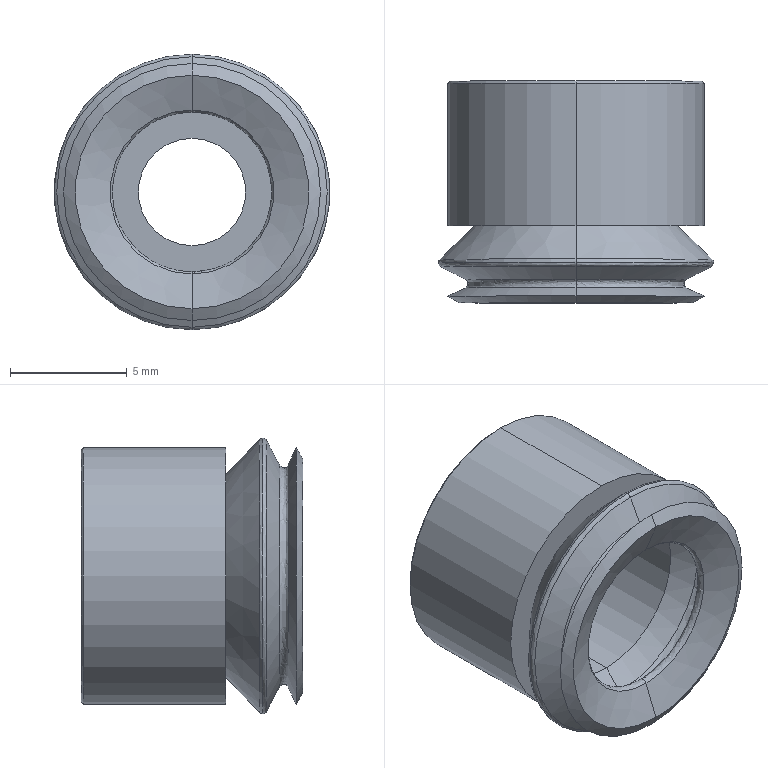Part | SolidWorks | features BaseBody 1 | 1 solid | 37 faces | box 11.8 x 9.5 x 11.8 mm | volume 493.379 mm3 | cone 16 | spline 12 | cylinder 6 | plane 3 | commonest cylinder face diameters 4.6 x2 7.8 x2 11 x2
STEP:
#1=CARTESIAN_POINT('',(0.,1.728,-5.9));
#2=VERTEX_POINT('',#1);
#3=CARTESIAN_POINT('',(0.,1.728,5.9));
#4=VERTEX_POINT('',#3);
#5=CARTESIAN_POINT('',(0.,1.728,0.));
#6=DIRECTION('',(0.,1.,0.));
#7=DIRECTION('',(0.,0.,1.));
#8=AXIS2_PLACEMENT_3D('',#5,#6,#7);
#9=CIRCLE('',#8,5.9);
#10=EDGE_CURVE('',#2,#4,#9,.T.);
#11=ORIENTED_EDGE('',*,*,#10,.F.);
#12=CARTESIAN_POINT('',(0.,1.551,-5.793));
#13=VERTEX_POINT('',#12);
#14=CARTESIAN_POINT('',(0.,1.728,-5.7));
#15=DIRECTION('',(-1.,0.,0.));
#16=DIRECTION('',(0.,0.,-1.));
#17=AXIS2_PLACEMENT_3D('',#14,#15,#16);
#18=CIRCLE('',#17,0.2);
#19=EDGE_CURVE('',#2,#13,#18,.T.);
#20=ORIENTED_EDGE('',*,*,#19,.T.);
#21=CARTESIAN_POINT('',(0.,1.551,5.793));
#22=VERTEX_POINT('',#21);
#23=CARTESIAN_POINT('',(0.,1.551,0.));
#24=DIRECTION('',(0.,1.,0.));
#25=DIRECTION('',(0.,0.,1.));
#26=AXIS2_PLACEMENT_3D('',#23,#24,#25);
#27=CIRCLE('',#26,5.793);
#28=EDGE_CURVE('',#13,#22,#27,.T.);
#29=ORIENTED_EDGE('',*,*,#28,.T.);
#30=CARTESIAN_POINT('',(0.,1.728,5.7));
#31=DIRECTION('',(1.,0.,0.));
#32=DIRECTION('',(0.,0.,1.));
#33=AXIS2_PLACEMENT_3D('',#30,#31,#32);
#34=CIRCLE('',#33,0.2);
#35=EDGE_CURVE('',#4,#22,#34,.T.);
#36=ORIENTED_EDGE('',*,*,#35,.F.);
#37=EDGE_LOOP('',(#11,#20,#29,#36));
#38=FACE_OUTER_BOUND('',#37,.T.);
#39=CARTESIAN_POINT('',(0.,1.728,-5.9));
#40=CARTESIAN_POINT('',(-11.8,1.728,-5.9));
#41=CARTESIAN_POINT('',(-11.8,1.728,5.9));
#42=CARTESIAN_POINT('',(0.,1.728,5.9));
#43=CARTESIAN_POINT('',(0.,1.652,-5.9));
#44=CARTESIAN_POINT('',(-11.8,1.652,-5.9));
#45=CARTESIAN_POINT('',(-11.8,1.652,5.9));
#46=CARTESIAN_POINT('',(0.,1.652,5.9));
#47=CARTESIAN_POINT('',(0.,1.586,-5.861));
#48=CARTESIAN_POINT('',(-11.721,1.586,-5.861));
#49=CARTESIAN_POINT('',(-11.721,1.586,5.861));
#50=CARTESIAN_POINT('',(0.,1.586,5.861));
#51=CARTESIAN_POINT('',(0.,1.551,-5.793));
#52=CARTESIAN_POINT('',(-11.586,1.551,-5.793));
#53=CARTESIAN_POINT('',(-11.586,1.551,5.793));
#54=CARTESIAN_POINT('',(0.,1.551,5.793));
#55=(BOUNDED_SURFACE()B_SPLINE_SURFACE(3,3,((#39,#40,#41,#42),(#43,#44,#45,#46),(#47,#48,#49,#50),(#51,#52,#53,#54)),.UNSPECIFIED.,.F.,.F.,.F.)B_SPLINE_SURFACE_WITH_KNOTS((4,4),(4,4),(0.,1.),(0.,1.),.UNSPECIFIED.)GEOMETRIC_REPRESENTATION_ITEM()RATIONAL_B_SPLINE_SURFACE(((1.,0.3333,0.3333,1.),(0.9036,0.3012,0.3012,0.9036),(0.9036,0.3012,0.3012,0.9036),(1.,0.3333,0.3333,1.)))REPRESENTATION_ITEM('')SURFACE());
#56=ADVANCED_FACE('',(#38),#55,.T.);
#57=CARTESIAN_POINT('',(0.,0.6361,-4.74));
#58=VERTEX_POINT('',#57);
#59=CARTESIAN_POINT('',(0.,0.6361,4.74));
#60=VERTEX_POINT('',#59);
#61=CARTESIAN_POINT('',(0.,0.6361,0.));
#62=DIRECTION('',(0.,-1.,0.));
#63=DIRECTION('',(0.,0.,1.));
#64=AXIS2_PLACEMENT_3D('',#61,#62,#63);
#65=CIRCLE('',#64,4.74);
#66=EDGE_CURVE('',#58,#60,#65,.T.);
#67=ORIENTED_EDGE('',*,*,#66,.F.);
#68=CARTESIAN_POINT('',(0.,0.9952,-4.73));
#69=VERTEX_POINT('',#68);
#70=CARTESIAN_POINT('',(0.,0.818,-4.823));
#71=DIRECTION('',(-1.,0.,0.));
#72=DIRECTION('',(0.,0.,-1.));
#73=AXIS2_PLACEMENT_3D('',#70,#71,#72);
#74=CIRCLE('',#73,0.2);
#75=EDGE_CURVE('',#58,#69,#74,.T.);
#76=ORIENTED_EDGE('',*,*,#75,.T.);
#77=CARTESIAN_POINT('',(0.,0.9952,4.73));
#78=VERTEX_POINT('',#77);
#79=CARTESIAN_POINT('',(0.,0.9952,0.));
#80=DIRECTION('',(0.,1.,0.));
#81=DIRECTION('',(0.,0.,1.));
#82=AXIS2_PLACEMENT_3D('',#79,#80,#81);
#83=CIRCLE('',#82,4.73);
#84=EDGE_CURVE('',#78,#69,#83,.T.);
#85=ORIENTED_EDGE('',*,*,#84,.F.);
#86=CARTESIAN_POINT('',(0.,0.818,4.823));
#87=DIRECTION('',(1.,0.,0.));
#88=DIRECTION('',(0.,0.,1.));
#89=AXIS2_PLACEMENT_3D('',#86,#87,#88);
#90=CIRCLE('',#89,0.2);
#91=EDGE_CURVE('',#60,#78,#90,.T.);
#92=ORIENTED_EDGE('',*,*,#91,.F.);
#93=EDGE_LOOP('',(#67,#76,#85,#92));
#94=FACE_OUTER_BOUND('',#93,.T.);
#95=CARTESIAN_POINT('',(0.,0.6361,4.74));
#96=CARTESIAN_POINT('',(9.48,0.6361,4.74));
#97=CARTESIAN_POINT('',(9.48,0.6361,-4.74));
#98=CARTESIAN_POINT('',(0.,0.6361,-4.74));
#99=CARTESIAN_POINT('',(0.,0.7156,4.566));
#100=CARTESIAN_POINT('',(9.132,0.7156,4.566));
#101=CARTESIAN_POINT('',(9.132,0.7156,-4.566));
#102=CARTESIAN_POINT('',(0.,0.7156,-4.566));
#103=CARTESIAN_POINT('',(0.,0.9066,4.561));
#104=CARTESIAN_POINT('',(9.122,0.9066,4.561));
#105=CARTESIAN_POINT('',(9.122,0.9066,-4.561));
#106=CARTESIAN_POINT('',(0.,0.9066,-4.561));
#107=CARTESIAN_POINT('',(0.,0.9952,4.73));
#108=CARTESIAN_POINT('',(9.461,0.9952,4.73));
#109=CARTESIAN_POINT('',(9.461,0.9952,-4.73));
#110=CARTESIAN_POINT('',(0.,0.9952,-4.73));
#111=(BOUNDED_SURFACE()B_SPLINE_SURFACE(3,3,((#95,#96,#97,#98),(#99,#100,#101,#102),(#103,#104,#105,#106),(#107,#108,#109,#110)),.UNSPECIFIED.,.F.,.F.,.F.)B_SPLINE_SURFACE_WITH_KNOTS((4,4),(4,4),(0.,1.),(0.,1.),.UNSPECIFIED.)GEOMETRIC_REPRESENTATION_ITEM()RATIONAL_B_SPLINE_SURFACE(((1.,0.3333,0.3333,1.),(0.6267,0.2089,0.2089,0.6267),(0.6267,0.2089,0.2089,0.6267),(1.,0.3333,0.3333,1.)))REPRESENTATION_ITEM('')SURFACE());
#112=ADVANCED_FACE('',(#94),#111,.F.);
#113=CARTESIAN_POINT('',(0.,2.2,4.732));
#114=VERTEX_POINT('',#113);
#115=CARTESIAN_POINT('',(0.,2.2,-4.732));
#116=VERTEX_POINT('',#115);
#117=CARTESIAN_POINT('',(0.,2.2,0.));
#118=DIRECTION('',(0.,1.,0.));
#119=DIRECTION('',(0.,0.,-1.));
#120=AXIS2_PLACEMENT_3D('',#117,#118,#119);
#121=CIRCLE('',#120,4.732);
#122=EDGE_CURVE('',#114,#116,#121,.T.);
#123=ORIENTED_EDGE('',*,*,#122,.T.);
#124=CARTESIAN_POINT('',(0.,1.912,-4.855));
#125=VERTEX_POINT('',#124);
#126=CARTESIAN_POINT('',(0.,1.912,-4.455));
#127=DIRECTION('',(-1.,0.,0.));
#128=DIRECTION('',(0.,0.,-1.));
#129=AXIS2_PLACEMENT_3D('',#126,#127,#128);
#130=CIRCLE('',#129,0.4);
#131=EDGE_CURVE('',#116,#125,#130,.T.);
#132=ORIENTED_EDGE('',*,*,#131,.T.);
#133=CARTESIAN_POINT('',(0.,1.912,4.855));
#134=VERTEX_POINT('',#133);
#135=CARTESIAN_POINT('',(0.,1.912,0.));
#136=DIRECTION('',(0.,1.,0.));
#137=DIRECTION('',(0.,0.,1.));
#138=AXIS2_PLACEMENT_3D('',#135,#136,#137);
#139=CIRCLE('',#138,4.855);
#140=EDGE_CURVE('',#134,#125,#139,.T.);
#141=ORIENTED_EDGE('',*,*,#140,.F.);
#142=CARTESIAN_POINT('',(0.,1.912,4.455));
#143=DIRECTION('',(1.,0.,0.));
#144=DIRECTION('',(0.,0.,1.));
#145=AXIS2_PLACEMENT_3D('',#142,#143,#144);
#146=CIRCLE('',#145,0.4);
#147=EDGE_CURVE('',#114,#134,#146,.T.);
#148=ORIENTED_EDGE('',*,*,#147,.F.);
#149=EDGE_LOOP('',(#123,#132,#141,#148));
#150=FACE_OUTER_BOUND('',#149,.T.);
#151=CARTESIAN_POINT('',(0.,2.2,4.732));
#152=CARTESIAN_POINT('',(9.464,2.2,4.732));
#153=CARTESIAN_POINT('',(9.464,2.2,-4.732));
#154=CARTESIAN_POINT('',(0.,2.2,-4.732));
#155=CARTESIAN_POINT('',(0.,2.124,4.811));
#156=CARTESIAN_POINT('',(9.623,2.124,4.811));
#157=CARTESIAN_POINT('',(9.623,2.124,-4.811));
#158=CARTESIAN_POINT('',(0.,2.124,-4.811));
#159=CARTESIAN_POINT('',(0.,2.022,4.855));
#160=CARTESIAN_POINT('',(9.709,2.022,4.855));
#161=CARTESIAN_POINT('',(9.709,2.022,-4.855));
#162=CARTESIAN_POINT('',(0.,2.022,-4.855));
#163=CARTESIAN_POINT('',(0.,1.912,4.855));
#164=CARTESIAN_POINT('',(9.709,1.912,4.855));
#165=CARTESIAN_POINT('',(9.709,1.912,-4.855));
#166=CARTESIAN_POINT('',(0.,1.912,-4.855));
#167=(BOUNDED_SURFACE()B_SPLINE_SURFACE(3,3,((#151,#152,#153,#154),(#155,#156,#157,#158),(#159,#160,#161,#162),(#163,#164,#165,#166)),.UNSPECIFIED.,.F.,.F.,.F.)B_SPLINE_SURFACE_WITH_KNOTS((4,4),(4,4),(0.,1.),(0.,1.),.UNSPECIFIED.)GEOMETRIC_REPRESENTATION_ITEM()RATIONAL_B_SPLINE_SURFACE(((1.,0.3333,0.3333,1.),(0.9467,0.3156,0.3156,0.9467),(0.9467,0.3156,0.3156,0.9467),(1.,0.3333,0.3333,1.)))REPRESENTATION_ITEM('')SURFACE());
#168=ADVANCED_FACE('',(#150),#167,.F.);
#169=CARTESIAN_POINT('',(0.,0.604,3.514));
#170=VERTEX_POINT('',#169);
#171=CARTESIAN_POINT('',(0.,0.604,-3.514));
#172=VERTEX_POINT('',#171);
#173=CARTESIAN_POINT('',(0.,0.604,0.));
#174=DIRECTION('',(0.,-1.,0.));
#175=DIRECTION('',(0.,0.,-1.));
#176=AXIS2_PLACEMENT_3D('',#173,#174,#175);
#177=CIRCLE('',#176,3.514);
#178=EDGE_CURVE('',#170,#172,#177,.T.);
#179=ORIENTED_EDGE('',*,*,#178,.T.);
#180=CARTESIAN_POINT('',(0.,0.956,-3.496));
#181=VERTEX_POINT('',#180);
#182=CARTESIAN_POINT('',(0.,0.7848,-3.599));
#183=DIRECTION('',(-1.,0.,0.));
#184=DIRECTION('',(0.,0.,-1.));
#185=AXIS2_PLACEMENT_3D('',#182,#183,#184);
#186=CIRCLE('',#185,0.2);
#187=EDGE_CURVE('',#172,#181,#186,.T.);
#188=ORIENTED_EDGE('',*,*,#187,.T.);
#189=CARTESIAN_POINT('',(0.,0.956,3.496));
#190=VERTEX_POINT('',#189);
#191=CARTESIAN_POINT('',(0.,0.956,0.));
#192=DIRECTION('',(0.,1.,0.));
#193=DIRECTION('',(0.,0.,1.));
#194=AXIS2_PLACEMENT_3D('',#191,#192,#193);
#195=CIRCLE('',#194,3.496);
#196=EDGE_CURVE('',#181,#190,#195,.T.);
#197=ORIENTED_EDGE('',*,*,#196,.T.);
#198=CARTESIAN_POINT('',(0.,0.7848,3.599));
#199=DIRECTION('',(1.,0.,0.));
#200=DIRECTION('',(0.,0.,1.));
#201=AXIS2_PLACEMENT_3D('',#198,#199,#200);
#202=CIRCLE('',#201,0.2);
#203=EDGE_CURVE('',#170,#190,#202,.T.);
#204=ORIENTED_EDGE('',*,*,#203,.F.);
#205=EDGE_LOOP('',(#179,#188,#197,#204));
#206=FACE_OUTER_BOUND('',#205,.T.);
#207=CARTESIAN_POINT('',(0.,0.604,-3.514));
#208=CARTESIAN_POINT('',(-7.028,0.604,-3.514));
#209=CARTESIAN_POINT('',(-7.028,0.604,3.514));
#210=CARTESIAN_POINT('',(0.,0.604,3.514));
#211=CARTESIAN_POINT('',(0.,0.6814,-3.35));
#212=CARTESIAN_POINT('',(-6.7,0.6814,-3.35));
#213=CARTESIAN_POINT('',(-6.7,0.6814,3.35));
#214=CARTESIAN_POINT('',(0.,0.6814,3.35));
#215=CARTESIAN_POINT('',(0.,0.8623,-3.341));
#216=CARTESIAN_POINT('',(-6.682,0.8623,-3.341));
#217=CARTESIAN_POINT('',(-6.682,0.8623,3.341));
#218=CARTESIAN_POINT('',(0.,0.8623,3.341));
#219=CARTESIAN_POINT('',(0.,0.956,-3.496));
#220=CARTESIAN_POINT('',(-6.992,0.956,-3.496));
#221=CARTESIAN_POINT('',(-6.992,0.956,3.496));
#222=CARTESIAN_POINT('',(0.,0.956,3.496));
#223=(BOUNDED_SURFACE()B_SPLINE_SURFACE(3,3,((#207,#208,#209,#210),(#211,#212,#213,#214),(#215,#216,#217,#218),(#219,#220,#221,#222)),.UNSPECIFIED.,.F.,.F.,.T.)B_SPLINE_SURFACE_WITH_KNOTS((4,4),(4,4),(0.,1.),(0.,1.),.UNSPECIFIED.)GEOMETRIC_REPRESENTATION_ITEM()RATIONAL_B_SPLINE_SURFACE(((1.,0.3333,0.3333,1.),(0.6486,0.2162,0.2162,0.6486),(0.6486,0.2162,0.2162,0.6486),(1.,0.3333,0.3333,1.)))REPRESENTATION_ITEM('')SURFACE());
#224=ADVANCED_FACE('',(#206),#223,.T.);
#225=ORIENTED_EDGE('',*,*,#140,.T.);
#226=CARTESIAN_POINT('',(0.,1.558,-4.641));
#227=VERTEX_POINT('',#226);
#228=CARTESIAN_POINT('',(0.,1.912,-4.455));
#229=DIRECTION('',(-1.,0.,0.));
#230=DIRECTION('',(0.,0.,-1.));
#231=AXIS2_PLACEMENT_3D('',#228,#229,#230);
#232=CIRCLE('',#231,0.4);
#233=EDGE_CURVE('',#125,#227,#232,.T.);
#234=ORIENTED_EDGE('',*,*,#233,.T.);
#235=CARTESIAN_POINT('',(0.,1.558,4.641));
#236=VERTEX_POINT('',#235);
#237=CARTESIAN_POINT('',(0.,1.558,0.));
#238=DIRECTION('',(0.,1.,0.));
#239=DIRECTION('',(0.,0.,1.));
#240=AXIS2_PLACEMENT_3D('',#237,#238,#239);
#241=CIRCLE('',#240,4.641);
#242=EDGE_CURVE('',#236,#227,#241,.T.);
#243=ORIENTED_EDGE('',*,*,#242,.F.);
#244=CARTESIAN_POINT('',(0.,1.912,4.455));
#245=DIRECTION('',(1.,0.,0.));
#246=DIRECTION('',(0.,0.,1.));
#247=AXIS2_PLACEMENT_3D('',#244,#245,#246);
#248=CIRCLE('',#247,0.4);
#249=EDGE_CURVE('',#134,#236,#248,.T.);
#250=ORIENTED_EDGE('',*,*,#249,.F.);
#251=EDGE_LOOP('',(#225,#234,#243,#250));
#252=FACE_OUTER_BOUND('',#251,.T.);
#253=CARTESIAN_POINT('',(0.,1.912,4.855));
#254=CARTESIAN_POINT('',(9.709,1.912,4.855));
#255=CARTESIAN_POINT('',(9.709,1.912,-4.855));
#256=CARTESIAN_POINT('',(0.,1.912,-4.855));
#257=CARTESIAN_POINT('',(0.,1.759,4.855));
#258=CARTESIAN_POINT('',(9.709,1.759,4.855));
#259=CARTESIAN_POINT('',(9.709,1.759,-4.855));
#260=CARTESIAN_POINT('',(0.,1.759,-4.855));
#261=CARTESIAN_POINT('',(0.,1.629,4.776));
#262=CARTESIAN_POINT('',(9.551,1.629,4.776));
#263=CARTESIAN_POINT('',(9.551,1.629,-4.776));
#264=CARTESIAN_POINT('',(0.,1.629,-4.776));
#265=CARTESIAN_POINT('',(0.,1.558,4.641));
#266=CARTESIAN_POINT('',(9.281,1.558,4.641));
#267=CARTESIAN_POINT('',(9.281,1.558,-4.641));
#268=CARTESIAN_POINT('',(0.,1.558,-4.641));
#269=(BOUNDED_SURFACE()B_SPLINE_SURFACE(3,3,((#253,#254,#255,#256),(#257,#258,#259,#260),(#261,#262,#263,#264),(#265,#266,#267,#268)),.UNSPECIFIED.,.F.,.F.,.F.)B_SPLINE_SURFACE_WITH_KNOTS((4,4),(4,4),(0.,1.),(0.,1.),.UNSPECIFIED.)GEOMETRIC_REPRESENTATION_ITEM()RATIONAL_B_SPLINE_SURFACE(((1.,0.3333,0.3333,1.),(0.904,0.3013,0.3013,0.904),(0.904,0.3013,0.3013,0.904),(1.,0.3333,0.3333,1.)))REPRESENTATION_ITEM('')SURFACE());
#270=ADVANCED_FACE('',(#252),#269,.F.);
#271=CARTESIAN_POINT('',(0.,1.873,-5.838));
#272=VERTEX_POINT('',#271);
#273=CARTESIAN_POINT('',(0.,1.873,5.838));
#274=VERTEX_POINT('',#273);
#275=CARTESIAN_POINT('',(0.,1.873,0.));
#276=DIRECTION('',(0.,1.,0.));
#277=DIRECTION('',(0.,0.,-1.));
#278=AXIS2_PLACEMENT_3D('',#275,#276,#277);
#279=CIRCLE('',#278,5.838);
#280=EDGE_CURVE('',#272,#274,#279,.T.);
#281=ORIENTED_EDGE('',*,*,#280,.F.);
#282=CARTESIAN_POINT('',(0.,1.728,-5.7));
#283=DIRECTION('',(-1.,0.,0.));
#284=DIRECTION('',(0.,0.,-1.));
#285=AXIS2_PLACEMENT_3D('',#282,#283,#284);
#286=CIRCLE('',#285,0.2);
#287=EDGE_CURVE('',#272,#2,#286,.T.);
#288=ORIENTED_EDGE('',*,*,#287,.T.);
#289=ORIENTED_EDGE('',*,*,#10,.T.);
#290=CARTESIAN_POINT('',(0.,1.728,5.7));
#291=DIRECTION('',(1.,0.,0.));
#292=DIRECTION('',(0.,0.,1.));
#293=AXIS2_PLACEMENT_3D('',#290,#291,#292);
#294=CIRCLE('',#293,0.2);
#295=EDGE_CURVE('',#274,#4,#294,.T.);
#296=ORIENTED_EDGE('',*,*,#295,.F.);
#297=EDGE_LOOP('',(#281,#288,#289,#296));
#298=FACE_OUTER_BOUND('',#297,.T.);
#299=CARTESIAN_POINT('',(0.,1.873,-5.838));
#300=CARTESIAN_POINT('',(-11.677,1.873,-5.838));
#301=CARTESIAN_POINT('',(-11.677,1.873,5.838));
#302=CARTESIAN_POINT('',(0.,1.873,5.838));
#303=CARTESIAN_POINT('',(0.,1.834,-5.878));
#304=CARTESIAN_POINT('',(-11.757,1.834,-5.878));
#305=CARTESIAN_POINT('',(-11.757,1.834,5.878));
#306=CARTESIAN_POINT('',(0.,1.834,5.878));
#307=CARTESIAN_POINT('',(0.,1.783,-5.9));
#308=CARTESIAN_POINT('',(-11.8,1.783,-5.9));
#309=CARTESIAN_POINT('',(-11.8,1.783,5.9));
#310=CARTESIAN_POINT('',(0.,1.783,5.9));
#311=CARTESIAN_POINT('',(0.,1.728,-5.9));
#312=CARTESIAN_POINT('',(-11.8,1.728,-5.9));
#313=CARTESIAN_POINT('',(-11.8,1.728,5.9));
#314=CARTESIAN_POINT('',(0.,1.728,5.9));
#315=(BOUNDED_SURFACE()B_SPLINE_SURFACE(3,3,((#299,#300,#301,#302),(#303,#304,#305,#306),(#307,#308,#309,#310),(#311,#312,#313,#314)),.UNSPECIFIED.,.F.,.F.,.F.)B_SPLINE_SURFACE_WITH_KNOTS((4,4),(4,4),(0.,1.),(0.,1.),.UNSPECIFIED.)GEOMETRIC_REPRESENTATION_ITEM()RATIONAL_B_SPLINE_SURFACE(((1.,0.3333,0.3333,1.),(0.9464,0.3155,0.3155,0.9464),(0.9464,0.3155,0.3155,0.9464),(1.,0.3333,0.3333,1.)))REPRESENTATION_ITEM('')SURFACE());
#316=ADVANCED_FACE('',(#298),#315,.T.);
#317=CARTESIAN_POINT('',(0.,9.4,-5.5));
#318=VERTEX_POINT('',#317);
#319=CARTESIAN_POINT('',(0.,9.4,5.5));
#320=VERTEX_POINT('',#319);
#321=CARTESIAN_POINT('',(0.,9.4,0.));
#322=DIRECTION('',(0.,-1.,0.));
#323=DIRECTION('',(0.,0.,-1.));
#324=AXIS2_PLACEMENT_3D('',#321,#322,#323);
#325=CIRCLE('',#324,5.5);
#326=EDGE_CURVE('',#318,#320,#325,.T.);
#327=ORIENTED_EDGE('',*,*,#326,.T.);
#328=CARTESIAN_POINT('',(0.,3.3,5.5));
#329=VERTEX_POINT('',#328);
#330=CARTESIAN_POINT('',(0.,50.,5.5));
#331=DIRECTION('',(0.,-1.,0.));
#332=VECTOR('',#331,1000.);
#333=LINE('',#330,#332);
#334=EDGE_CURVE('',#320,#329,#333,.T.);
#335=ORIENTED_EDGE('',*,*,#334,.T.);
#336=CARTESIAN_POINT('',(0.,3.3,-5.5));
#337=VERTEX_POINT('',#336);
#338=CARTESIAN_POINT('',(0.,3.3,0.));
#339=DIRECTION('',(0.,1.,0.));
#340=DIRECTION('',(0.,0.,-1.));
#341=AXIS2_PLACEMENT_3D('',#338,#339,#340);
#342=CIRCLE('',#341,5.5);
#343=EDGE_CURVE('',#329,#337,#342,.T.);
#344=ORIENTED_EDGE('',*,*,#343,.T.);
#345=CARTESIAN_POINT('',(0.,50.,-5.5));
#346=DIRECTION('',(0.,-1.,0.));
#347=VECTOR('',#346,1000.);
#348=LINE('',#345,#347);
#349=EDGE_CURVE('',#318,#337,#348,.T.);
#350=ORIENTED_EDGE('',*,*,#349,.F.);
#351=EDGE_LOOP('',(#327,#335,#344,#350));
#352=FACE_OUTER_BOUND('',#351,.T.);
#353=CARTESIAN_POINT('',(0.,50.,0.));
#354=DIRECTION('',(0.,-1.,0.));
#355=DIRECTION('',(0.,0.,-1.));
#356=AXIS2_PLACEMENT_3D('',#353,#354,#355);
#357=CYLINDRICAL_SURFACE('',#356,5.5);
#358=ADVANCED_FACE('',(#352),#357,.T.);
#359=CARTESIAN_POINT('',(0.,9.5,-5.4));
#360=VERTEX_POINT('',#359);
#361=CARTESIAN_POINT('',(0.,9.5,5.4));
#362=VERTEX_POINT('',#361);
#363=CARTESIAN_POINT('',(0.,9.5,0.));
#364=DIRECTION('',(0.,-1.,0.));
#365=DIRECTION('',(0.,0.,-1.));
#366=AXIS2_PLACEMENT_3D('',#363,#364,#365);
#367=CIRCLE('',#366,5.4);
#368=EDGE_CURVE('',#360,#362,#367,.T.);
#369=ORIENTED_EDGE('',*,*,#368,.T.);
#370=CARTESIAN_POINT('',(0.,9.4,5.5));
#371=DIRECTION('',(0.,-0.7071,0.7071));
#372=VECTOR('',#371,1000.);
#373=LINE('',#370,#372);
#374=EDGE_CURVE('',#362,#320,#373,.T.);
#375=ORIENTED_EDGE('',*,*,#374,.T.);
#376=ORIENTED_EDGE('',*,*,#326,.F.);
#377=CARTESIAN_POINT('',(0.,9.4,-5.5));
#378=DIRECTION('',(0.,-0.7071,-0.7071));
#379=VECTOR('',#378,1000.);
#380=LINE('',#377,#379);
#381=EDGE_CURVE('',#360,#318,#380,.T.);
#382=ORIENTED_EDGE('',*,*,#381,.F.);
#383=EDGE_LOOP('',(#369,#375,#376,#382));
#384=FACE_OUTER_BOUND('',#383,.T.);
#385=CARTESIAN_POINT('',(0.,9.4,0.));
#386=DIRECTION('',(0.,-1.,0.));
#387=DIRECTION('',(0.,0.,-1.));
#388=AXIS2_PLACEMENT_3D('',#385,#386,#387);
#389=CONICAL_SURFACE('',#388,5.5,0.7854);
#390=ADVANCED_FACE('',(#384),#389,.T.);
#391=CARTESIAN_POINT('',(0.,3.3,4.347));
#392=VERTEX_POINT('',#391);
#393=CARTESIAN_POINT('',(0.,3.3,-4.347));
#394=VERTEX_POINT('',#393);
#395=CARTESIAN_POINT('',(0.,3.3,0.));
#396=DIRECTION('',(0.,1.,0.));
#397=DIRECTION('',(0.,0.,-1.));
#398=AXIS2_PLACEMENT_3D('',#395,#396,#397);
#399=CIRCLE('',#398,4.347);
#400=EDGE_CURVE('',#392,#394,#399,.T.);
#401=ORIENTED_EDGE('',*,*,#400,.F.);
#402=CARTESIAN_POINT('',(0.,1.873,5.838));
#403=DIRECTION('',(0.,-0.6914,0.7224));
#404=VECTOR('',#403,1000.);
#405=LINE('',#402,#404);
#406=EDGE_CURVE('',#392,#274,#405,.T.);
#407=ORIENTED_EDGE('',*,*,#406,.T.);
#408=CARTESIAN_POINT('',(0.,1.873,0.));
#409=DIRECTION('',(0.,1.,0.));
#410=DIRECTION('',(0.,0.,-1.));
#411=AXIS2_PLACEMENT_3D('',#408,#409,#410);
#412=CIRCLE('',#411,5.838);
#413=EDGE_CURVE('',#274,#272,#412,.T.);
#414=ORIENTED_EDGE('',*,*,#413,.T.);
#415=CARTESIAN_POINT('',(0.,1.873,-5.838));
#416=DIRECTION('',(0.,-0.6914,-0.7224));
#417=VECTOR('',#416,1000.);
#418=LINE('',#415,#417);
#419=EDGE_CURVE('',#394,#272,#418,.T.);
#420=ORIENTED_EDGE('',*,*,#419,.F.);
#421=EDGE_LOOP('',(#401,#407,#414,#420));
#422=FACE_OUTER_BOUND('',#421,.T.);
#423=CARTESIAN_POINT('',(0.,1.873,0.));
#424=DIRECTION('',(0.,-1.,0.));
#425=DIRECTION('',(0.,0.,-1.));
#426=AXIS2_PLACEMENT_3D('',#423,#424,#425);
#427=CONICAL_SURFACE('',#426,5.838,0.8073);
#428=ADVANCED_FACE('',(#422),#427,.T.);
#429=CARTESIAN_POINT('',(0.,9.5,2.3));
#430=VERTEX_POINT('',#429);
#431=CARTESIAN_POINT('',(0.,9.5,-2.3));
#432=VERTEX_POINT('',#431);
#433=CARTESIAN_POINT('',(0.,9.5,0.));
#434=DIRECTION('',(0.,-1.,0.));
#435=DIRECTION('',(0.,0.,-1.));
#436=AXIS2_PLACEMENT_3D('',#433,#434,#435);
#437=CIRCLE('',#436,2.3);
#438=EDGE_CURVE('',#430,#432,#437,.T.);
#439=ORIENTED_EDGE('',*,*,#438,.F.);
#440=CARTESIAN_POINT('',(0.,6.,2.3));
#441=VERTEX_POINT('',#440);
#442=CARTESIAN_POINT('',(0.,50.,2.3));
#443=DIRECTION('',(0.,-1.,0.));
#444=VECTOR('',#443,1000.);
#445=LINE('',#442,#444);
#446=EDGE_CURVE('',#430,#441,#445,.T.);
#447=ORIENTED_EDGE('',*,*,#446,.T.);
#448=CARTESIAN_POINT('',(0.,6.,-2.3));
#449=VERTEX_POINT('',#448);
#450=CARTESIAN_POINT('',(0.,6.,0.));
#451=DIRECTION('',(0.,1.,0.));
#452=DIRECTION('',(0.,0.,-1.));
#453=AXIS2_PLACEMENT_3D('',#450,#451,#452);
#454=CIRCLE('',#453,2.3);
#455=EDGE_CURVE('',#449,#441,#454,.T.);
#456=ORIENTED_EDGE('',*,*,#455,.F.);
#457=CARTESIAN_POINT('',(0.,50.,-2.3));
#458=DIRECTION('',(0.,-1.,0.));
#459=VECTOR('',#458,1000.);
#460=LINE('',#457,#459);
#461=EDGE_CURVE('',#432,#449,#460,.T.);
#462=ORIENTED_EDGE('',*,*,#461,.F.);
#463=EDGE_LOOP('',(#439,#447,#456,#462));
#464=FACE_OUTER_BOUND('',#463,.T.);
#465=CARTESIAN_POINT('',(0.,50.,0.));
#466=DIRECTION('',(0.,-1.,0.));
#467=DIRECTION('',(0.,0.,-1.));
#468=AXIS2_PLACEMENT_3D('',#465,#466,#467);
#469=CYLINDRICAL_SURFACE('',#468,2.3);
#470=ADVANCED_FACE('',(#464),#469,.F.);
#471=ORIENTED_EDGE('',*,*,#287,.F.);
#472=ORIENTED_EDGE('',*,*,#413,.F.);
#473=ORIENTED_EDGE('',*,*,#295,.T.);
#474=CARTESIAN_POINT('',(0.,1.728,0.));
#475=DIRECTION('',(0.,1.,0.));
#476=DIRECTION('',(0.,0.,1.));
#477=AXIS2_PLACEMENT_3D('',#474,#475,#476);
#478=CIRCLE('',#477,5.9);
#479=EDGE_CURVE('',#4,#2,#478,.T.);
#480=ORIENTED_EDGE('',*,*,#479,.T.);
#481=EDGE_LOOP('',(#471,#472,#473,#480));
#482=FACE_OUTER_BOUND('',#481,.T.);
#483=CARTESIAN_POINT('',(0.,1.873,5.838));
#484=CARTESIAN_POINT('',(11.677,1.873,5.838));
#485=CARTESIAN_POINT('',(11.677,1.873,-5.838));
#486=CARTESIAN_POINT('',(0.,1.873,-5.838));
#487=CARTESIAN_POINT('',(0.,1.834,5.878));
#488=CARTESIAN_POINT('',(11.757,1.834,5.878));
#489=CARTESIAN_POINT('',(11.757,1.834,-5.878));
#490=CARTESIAN_POINT('',(0.,1.834,-5.878));
#491=CARTESIAN_POINT('',(0.,1.783,5.9));
#492=CARTESIAN_POINT('',(11.8,1.783,5.9));
#493=CARTESIAN_POINT('',(11.8,1.783,-5.9));
#494=CARTESIAN_POINT('',(0.,1.783,-5.9));
#495=CARTESIAN_POINT('',(0.,1.728,5.9));
#496=CARTESIAN_POINT('',(11.8,1.728,5.9));
#497=CARTESIAN_POINT('',(11.8,1.728,-5.9));
#498=CARTESIAN_POINT('',(0.,1.728,-5.9));
#499=(BOUNDED_SURFACE()B_SPLINE_SURFACE(3,3,((#483,#484,#485,#486),(#487,#488,#489,#490),(#491,#492,#493,#494),(#495,#496,#497,#498)),.UNSPECIFIED.,.F.,.F.,.F.)B_SPLINE_SURFACE_WITH_KNOTS((4,4),(4,4),(0.,1.),(0.,1.),.UNSPECIFIED.)GEOMETRIC_REPRESENTATION_ITEM()RATIONAL_B_SPLINE_SURFACE(((1.,0.3333,0.3333,1.),(0.9464,0.3155,0.3155,0.9464),(0.9464,0.3155,0.3155,0.9464),(1.,0.3333,0.3333,1.)))REPRESENTATION_ITEM('')SURFACE());
#500=ADVANCED_FACE('',(#482),#499,.T.);
#501=ORIENTED_EDGE('',*,*,#84,.T.);
#502=CARTESIAN_POINT('',(0.,1.551,-5.793));
#503=DIRECTION('',(0.,0.4635,-0.8861));
#504=VECTOR('',#503,1000.);
#505=LINE('',#502,#504);
#506=EDGE_CURVE('',#69,#13,#505,.T.);
#507=ORIENTED_EDGE('',*,*,#506,.T.);
#508=CARTESIAN_POINT('',(0.,1.551,0.));
#509=DIRECTION('',(0.,1.,0.));
#510=DIRECTION('',(0.,0.,1.));
#511=AXIS2_PLACEMENT_3D('',#508,#509,#510);
#512=CIRCLE('',#511,5.793);
#513=EDGE_CURVE('',#22,#13,#512,.T.);
#514=ORIENTED_EDGE('',*,*,#513,.F.);
#515=CARTESIAN_POINT('',(0.,1.551,5.793));
#516=DIRECTION('',(0.,0.4635,0.8861));
#517=VECTOR('',#516,1000.);
#518=LINE('',#515,#517);
#519=EDGE_CURVE('',#78,#22,#518,.T.);
#520=ORIENTED_EDGE('',*,*,#519,.F.);
#521=EDGE_LOOP('',(#501,#507,#514,#520));
#522=FACE_OUTER_BOUND('',#521,.T.);
#523=CARTESIAN_POINT('',(0.,1.551,0.));
#524=DIRECTION('',(0.,1.,0.));
#525=DIRECTION('',(0.,0.,1.));
#526=AXIS2_PLACEMENT_3D('',#523,#524,#525);
#527=CONICAL_SURFACE('',#526,5.793,1.089);
#528=ADVANCED_FACE('',(#522),#527,.T.);
#529=CARTESIAN_POINT('',(0.,6.,3.9));
#530=VERTEX_POINT('',#529);
#531=CARTESIAN_POINT('',(0.,6.,-3.9));
#532=VERTEX_POINT('',#531);
#533=CARTESIAN_POINT('',(0.,6.,0.));
#534=DIRECTION('',(0.,-1.,0.));
#535=DIRECTION('',(0.,0.,-1.));
#536=AXIS2_PLACEMENT_3D('',#533,#534,#535);
#537=CIRCLE('',#536,3.9);
#538=EDGE_CURVE('',#530,#532,#537,.T.);
#539=ORIENTED_EDGE('',*,*,#538,.F.);
#540=CARTESIAN_POINT('',(0.,3.,3.9));
#541=VERTEX_POINT('',#540);
#542=CARTESIAN_POINT('',(0.,50.,3.9));
#543=DIRECTION('',(0.,-1.,0.));
#544=VECTOR('',#543,1000.);
#545=LINE('',#542,#544);
#546=EDGE_CURVE('',#530,#541,#545,.T.);
#547=ORIENTED_EDGE('',*,*,#546,.T.);
#548=CARTESIAN_POINT('',(0.,3.,-3.9));
#549=VERTEX_POINT('',#548);
#550=CARTESIAN_POINT('',(0.,3.,0.));
#551=DIRECTION('',(0.,1.,0.));
#552=DIRECTION('',(0.,0.,-1.));
#553=AXIS2_PLACEMENT_3D('',#550,#551,#552);
#554=CIRCLE('',#553,3.9);
#555=EDGE_CURVE('',#549,#541,#554,.T.);
#556=ORIENTED_EDGE('',*,*,#555,.F.);
#557=CARTESIAN_POINT('',(0.,50.,-3.9));
#558=DIRECTION('',(0.,-1.,0.));
#559=VECTOR('',#558,1000.);
#560=LINE('',#557,#559);
#561=EDGE_CURVE('',#532,#549,#560,.T.);
#562=ORIENTED_EDGE('',*,*,#561,.F.);
#563=EDGE_LOOP('',(#539,#547,#556,#562));
#564=FACE_OUTER_BOUND('',#563,.T.);
#565=CARTESIAN_POINT('',(0.,50.,0.));
#566=DIRECTION('',(0.,-1.,0.));
#567=DIRECTION('',(0.,0.,-1.));
#568=AXIS2_PLACEMENT_3D('',#565,#566,#567);
#569=CYLINDRICAL_SURFACE('',#568,3.9);
#570=ADVANCED_FACE('',(#564),#569,.F.);
#571=ORIENTED_EDGE('',*,*,#555,.T.);
#572=CARTESIAN_POINT('',(0.,2.2,4.732));
#573=DIRECTION('',(0.,-0.6931,0.7208));
#574=VECTOR('',#573,1000.);
#575=LINE('',#572,#574);
#576=EDGE_CURVE('',#541,#114,#575,.T.);
#577=ORIENTED_EDGE('',*,*,#576,.T.);
#578=CARTESIAN_POINT('',(0.,2.2,0.));
#579=DIRECTION('',(0.,1.,0.));
#580=DIRECTION('',(0.,0.,-1.));
#581=AXIS2_PLACEMENT_3D('',#578,#579,#580);
#582=CIRCLE('',#581,4.732);
#583=EDGE_CURVE('',#116,#114,#582,.T.);
#584=ORIENTED_EDGE('',*,*,#583,.F.);
#585=CARTESIAN_POINT('',(0.,2.2,-4.732));
#586=DIRECTION('',(0.,-0.6931,-0.7208));
#587=VECTOR('',#586,1000.);
#588=LINE('',#585,#587);
#589=EDGE_CURVE('',#549,#116,#588,.T.);
#590=ORIENTED_EDGE('',*,*,#589,.F.);
#591=EDGE_LOOP('',(#571,#577,#584,#590));
#592=FACE_OUTER_BOUND('',#591,.T.);
#593=CARTESIAN_POINT('',(0.,2.2,0.));
#594=DIRECTION('',(0.,-1.,0.));
#595=DIRECTION('',(0.,0.,-1.));
#596=AXIS2_PLACEMENT_3D('',#593,#594,#595);
#597=CONICAL_SURFACE('',#596,4.732,0.805);
#598=ADVANCED_FACE('',(#592),#597,.F.);
#599=ORIENTED_EDGE('',*,*,#66,.T.);
#600=CARTESIAN_POINT('',(0.,0.288,5.5));
#601=VERTEX_POINT('',#600);
#602=CARTESIAN_POINT('',(0.,0.288,5.5));
#603=DIRECTION('',(0.,-0.4163,0.9092));
#604=VECTOR('',#603,1000.);
#605=LINE('',#602,#604);
#606=EDGE_CURVE('',#60,#601,#605,.T.);
#607=ORIENTED_EDGE('',*,*,#606,.T.);
#608=CARTESIAN_POINT('',(0.,0.288,-5.5));
#609=VERTEX_POINT('',#608);
#610=CARTESIAN_POINT('',(0.,0.288,0.));
#611=DIRECTION('',(0.,1.,0.));
#612=DIRECTION('',(0.,0.,-1.));
#613=AXIS2_PLACEMENT_3D('',#610,#611,#612);
#614=CIRCLE('',#613,5.5);
#615=EDGE_CURVE('',#601,#609,#614,.T.);
#616=ORIENTED_EDGE('',*,*,#615,.T.);
#617=CARTESIAN_POINT('',(0.,0.288,-5.5));
#618=DIRECTION('',(0.,-0.4163,-0.9092));
#619=VECTOR('',#618,1000.);
#620=LINE('',#617,#619);
#621=EDGE_CURVE('',#58,#609,#620,.T.);
#622=ORIENTED_EDGE('',*,*,#621,.F.);
#623=EDGE_LOOP('',(#599,#607,#616,#622));
#624=FACE_OUTER_BOUND('',#623,.T.);
#625=CARTESIAN_POINT('',(0.,0.288,0.));
#626=DIRECTION('',(0.,-1.,0.));
#627=DIRECTION('',(0.,0.,-1.));
#628=AXIS2_PLACEMENT_3D('',#625,#626,#627);
#629=CONICAL_SURFACE('',#628,5.5,1.141);
#630=ADVANCED_FACE('',(#624),#629,.T.);
#631=ORIENTED_EDGE('',*,*,#233,.F.);
#632=CARTESIAN_POINT('',(0.,1.912,0.));
#633=DIRECTION('',(0.,1.,0.));
#634=DIRECTION('',(0.,0.,1.));
#635=AXIS2_PLACEMENT_3D('',#632,#633,#634);
#636=CIRCLE('',#635,4.855);
#637=EDGE_CURVE('',#125,#134,#636,.T.);
#638=ORIENTED_EDGE('',*,*,#637,.T.);
#639=ORIENTED_EDGE('',*,*,#249,.T.);
#640=CARTESIAN_POINT('',(0.,1.558,0.));
#641=DIRECTION('',(0.,1.,0.));
#642=DIRECTION('',(0.,0.,1.));
#643=AXIS2_PLACEMENT_3D('',#640,#641,#642);
#644=CIRCLE('',#643,4.641);
#645=EDGE_CURVE('',#227,#236,#644,.T.);
#646=ORIENTED_EDGE('',*,*,#645,.F.);
#647=EDGE_LOOP('',(#631,#638,#639,#646));
#648=FACE_OUTER_BOUND('',#647,.T.);
#649=CARTESIAN_POINT('',(0.,1.912,-4.855));
#650=CARTESIAN_POINT('',(-9.709,1.912,-4.855));
#651=CARTESIAN_POINT('',(-9.709,1.912,4.855));
#652=CARTESIAN_POINT('',(0.,1.912,4.855));
#653=CARTESIAN_POINT('',(0.,1.759,-4.855));
#654=CARTESIAN_POINT('',(-9.709,1.759,-4.855));
#655=CARTESIAN_POINT('',(-9.709,1.759,4.855));
#656=CARTESIAN_POINT('',(0.,1.759,4.855));
#657=CARTESIAN_POINT('',(0.,1.629,-4.776));
#658=CARTESIAN_POINT('',(-9.551,1.629,-4.776));
#659=CARTESIAN_POINT('',(-9.551,1.629,4.776));
#660=CARTESIAN_POINT('',(0.,1.629,4.776));
#661=CARTESIAN_POINT('',(0.,1.558,-4.641));
#662=CARTESIAN_POINT('',(-9.281,1.558,-4.641));
#663=CARTESIAN_POINT('',(-9.281,1.558,4.641));
#664=CARTESIAN_POINT('',(0.,1.558,4.641));
#665=(BOUNDED_SURFACE()B_SPLINE_SURFACE(3,3,((#649,#650,#651,#652),(#653,#654,#655,#656),(#657,#658,#659,#660),(#661,#662,#663,#664)),.UNSPECIFIED.,.F.,.F.,.F.)B_SPLINE_SURFACE_WITH_KNOTS((4,4),(4,4),(0.,1.),(0.,1.),.UNSPECIFIED.)GEOMETRIC_REPRESENTATION_ITEM()RATIONAL_B_SPLINE_SURFACE(((1.,0.3333,0.3333,1.),(0.904,0.3013,0.3013,0.904),(0.904,0.3013,0.3013,0.904),(1.,0.3333,0.3333,1.)))REPRESENTATION_ITEM('')SURFACE());
#666=ADVANCED_FACE('',(#648),#665,.F.);
#667=CARTESIAN_POINT('',(0.,0.,5.));
#668=VERTEX_POINT('',#667);
#669=CARTESIAN_POINT('',(0.,0.,-5.));
#670=VERTEX_POINT('',#669);
#671=CARTESIAN_POINT('',(0.,0.,0.));
#672=DIRECTION('',(0.,1.,0.));
#673=DIRECTION('',(0.,0.,1.));
#674=AXIS2_PLACEMENT_3D('',#671,#672,#673);
#675=CIRCLE('',#674,5.);
#676=EDGE_CURVE('',#668,#670,#675,.T.);
#677=ORIENTED_EDGE('',*,*,#676,.T.);
#678=CARTESIAN_POINT('',(0.,0.288,-5.5));
#679=DIRECTION('',(0.,0.4991,-0.8665));
#680=VECTOR('',#679,1000.);
#681=LINE('',#678,#680);
#682=EDGE_CURVE('',#670,#609,#681,.T.);
#683=ORIENTED_EDGE('',*,*,#682,.T.);
#684=ORIENTED_EDGE('',*,*,#615,.F.);
#685=CARTESIAN_POINT('',(0.,0.288,5.5));
#686=DIRECTION('',(0.,0.4991,0.8665));
#687=VECTOR('',#686,1000.);
#688=LINE('',#685,#687);
#689=EDGE_CURVE('',#668,#601,#688,.T.);
#690=ORIENTED_EDGE('',*,*,#689,.F.);
#691=EDGE_LOOP('',(#677,#683,#684,#690));
#692=FACE_OUTER_BOUND('',#691,.T.);
#693=CARTESIAN_POINT('',(0.,0.288,0.));
#694=DIRECTION('',(0.,1.,0.));
#695=DIRECTION('',(0.,0.,1.));
#696=AXIS2_PLACEMENT_3D('',#693,#694,#695);
#697=CONICAL_SURFACE('',#696,5.5,1.048);
#698=ADVANCED_FACE('',(#692),#697,.T.);
#699=ORIENTED_EDGE('',*,*,#196,.F.);
#700=CARTESIAN_POINT('',(0.,1.558,-4.641));
#701=DIRECTION('',(0.,0.4654,-0.8851));
#702=VECTOR('',#701,1000.);
#703=LINE('',#700,#702);
#704=EDGE_CURVE('',#181,#227,#703,.T.);
#705=ORIENTED_EDGE('',*,*,#704,.T.);
#706=ORIENTED_EDGE('',*,*,#645,.T.);
#707=CARTESIAN_POINT('',(0.,1.558,4.641));
#708=DIRECTION('',(0.,0.4654,0.8851));
#709=VECTOR('',#708,1000.);
#710=LINE('',#707,#709);
#711=EDGE_CURVE('',#190,#236,#710,.T.);
#712=ORIENTED_EDGE('',*,*,#711,.F.);
#713=EDGE_LOOP('',(#699,#705,#706,#712));
#714=FACE_OUTER_BOUND('',#713,.T.);
#715=CARTESIAN_POINT('',(0.,1.558,0.));
#716=DIRECTION('',(0.,1.,0.));
#717=DIRECTION('',(0.,0.,1.));
#718=AXIS2_PLACEMENT_3D('',#715,#716,#717);
#719=CONICAL_SURFACE('',#718,4.641,1.087);
#720=ADVANCED_FACE('',(#714),#719,.F.);
#721=ORIENTED_EDGE('',*,*,#178,.F.);
#722=CARTESIAN_POINT('',(0.,0.,5.));
#723=DIRECTION('',(0.,-0.3765,0.9264));
#724=VECTOR('',#723,1000.);
#725=LINE('',#722,#724);
#726=EDGE_CURVE('',#170,#668,#725,.T.);
#727=ORIENTED_EDGE('',*,*,#726,.T.);
#728=CARTESIAN_POINT('',(0.,0.,0.));
#729=DIRECTION('',(0.,1.,0.));
#730=DIRECTION('',(0.,0.,1.));
#731=AXIS2_PLACEMENT_3D('',#728,#729,#730);
#732=CIRCLE('',#731,5.);
#733=EDGE_CURVE('',#670,#668,#732,.T.);
#734=ORIENTED_EDGE('',*,*,#733,.F.);
#735=CARTESIAN_POINT('',(0.,0.,-5.));
#736=DIRECTION('',(0.,-0.3765,-0.9264));
#737=VECTOR('',#736,1000.);
#738=LINE('',#735,#737);
#739=EDGE_CURVE('',#172,#670,#738,.T.);
#740=ORIENTED_EDGE('',*,*,#739,.F.);
#741=EDGE_LOOP('',(#721,#727,#734,#740));
#742=FACE_OUTER_BOUND('',#741,.T.);
#743=CARTESIAN_POINT('',(0.,0.,0.));
#744=DIRECTION('',(0.,-1.,0.));
#745=DIRECTION('',(0.,0.,-1.));
#746=AXIS2_PLACEMENT_3D('',#743,#744,#745);
#747=CONICAL_SURFACE('',#746,5.,1.185);
#748=ADVANCED_FACE('',(#742),#747,.F.);
#749=ORIENTED_EDGE('',*,*,#334,.F.);
#750=CARTESIAN_POINT('',(0.,9.4,0.));
#751=DIRECTION('',(0.,-1.,0.));
#752=DIRECTION('',(0.,0.,-1.));
#753=AXIS2_PLACEMENT_3D('',#750,#751,#752);
#754=CIRCLE('',#753,5.5);
#755=EDGE_CURVE('',#320,#318,#754,.T.);
#756=ORIENTED_EDGE('',*,*,#755,.T.);
#757=ORIENTED_EDGE('',*,*,#349,.T.);
#758=CARTESIAN_POINT('',(0.,3.3,0.));
#759=DIRECTION('',(0.,1.,0.));
#760=DIRECTION('',(0.,0.,-1.));
#761=AXIS2_PLACEMENT_3D('',#758,#759,#760);
#762=CIRCLE('',#761,5.5);
#763=EDGE_CURVE('',#337,#329,#762,.T.);
#764=ORIENTED_EDGE('',*,*,#763,.T.);
#765=EDGE_LOOP('',(#749,#756,#757,#764));
#766=FACE_OUTER_BOUND('',#765,.T.);
#767=CARTESIAN_POINT('',(0.,50.,0.));
#768=DIRECTION('',(0.,-1.,0.));
#769=DIRECTION('',(0.,0.,-1.));
#770=AXIS2_PLACEMENT_3D('',#767,#768,#769);
#771=CYLINDRICAL_SURFACE('',#770,5.5);
#772=ADVANCED_FACE('',(#766),#771,.T.);
#773=ORIENTED_EDGE('',*,*,#374,.F.);
#774=CARTESIAN_POINT('',(0.,9.5,0.));
#775=DIRECTION('',(0.,-1.,0.));
#776=DIRECTION('',(0.,0.,-1.));
#777=AXIS2_PLACEMENT_3D('',#774,#775,#776);
#778=CIRCLE('',#777,5.4);
#779=EDGE_CURVE('',#362,#360,#778,.T.);
#780=ORIENTED_EDGE('',*,*,#779,.T.);
#781=ORIENTED_EDGE('',*,*,#381,.T.);
#782=ORIENTED_EDGE('',*,*,#755,.F.);
#783=EDGE_LOOP('',(#773,#780,#781,#782));
#784=FACE_OUTER_BOUND('',#783,.T.);
#785=CARTESIAN_POINT('',(0.,9.4,0.));
#786=DIRECTION('',(0.,-1.,0.));
#787=DIRECTION('',(0.,0.,-1.));
#788=AXIS2_PLACEMENT_3D('',#785,#786,#787);
#789=CONICAL_SURFACE('',#788,5.5,0.7854);
#790=ADVANCED_FACE('',(#784),#789,.T.);
#791=ORIENTED_EDGE('',*,*,#763,.F.);
#792=ORIENTED_EDGE('',*,*,#343,.F.);
#793=EDGE_LOOP('',(#791,#792));
#794=FACE_OUTER_BOUND('',#793,.T.);
#795=CARTESIAN_POINT('',(0.,3.3,0.));
#796=DIRECTION('',(0.,1.,0.));
#797=DIRECTION('',(0.,0.,-1.));
#798=AXIS2_PLACEMENT_3D('',#795,#796,#797);
#799=CIRCLE('',#798,4.347);
#800=EDGE_CURVE('',#394,#392,#799,.T.);
#801=ORIENTED_EDGE('',*,*,#800,.T.);
#802=ORIENTED_EDGE('',*,*,#400,.T.);
#803=EDGE_LOOP('',(#801,#802));
#804=FACE_BOUND('',#803,.T.);
#805=CARTESIAN_POINT('',(0.,3.3,5.5));
#806=DIRECTION('',(0.,-1.,0.));
#807=DIRECTION('',(0.,0.,-1.));
#808=AXIS2_PLACEMENT_3D('',#805,#806,#807);
#809=PLANE('',#808);
#810=ADVANCED_FACE('',(#794,#804),#809,.T.);
#811=CARTESIAN_POINT('',(0.,9.5,0.));
#812=DIRECTION('',(0.,-1.,0.));
#813=DIRECTION('',(0.,0.,-1.));
#814=AXIS2_PLACEMENT_3D('',#811,#812,#813);
#815=CIRCLE('',#814,2.3);
#816=EDGE_CURVE('',#432,#430,#815,.T.);
#817=ORIENTED_EDGE('',*,*,#816,.T.);
#818=ORIENTED_EDGE('',*,*,#438,.T.);
#819=EDGE_LOOP('',(#817,#818));
#820=FACE_BOUND('',#819,.T.);
#821=ORIENTED_EDGE('',*,*,#368,.F.);
#822=ORIENTED_EDGE('',*,*,#779,.F.);
#823=EDGE_LOOP('',(#821,#822));
#824=FACE_OUTER_BOUND('',#823,.T.);
#825=CARTESIAN_POINT('',(0.,9.5,2.3));
#826=DIRECTION('',(0.,1.,0.));
#827=DIRECTION('',(0.,0.,1.));
#828=AXIS2_PLACEMENT_3D('',#825,#826,#827);
#829=PLANE('',#828);
#830=ADVANCED_FACE('',(#820,#824),#829,.T.);
#831=ORIENTED_EDGE('',*,*,#406,.F.);
#832=ORIENTED_EDGE('',*,*,#800,.F.);
#833=ORIENTED_EDGE('',*,*,#419,.T.);
#834=ORIENTED_EDGE('',*,*,#280,.T.);
#835=EDGE_LOOP('',(#831,#832,#833,#834));
#836=FACE_OUTER_BOUND('',#835,.T.);
#837=CARTESIAN_POINT('',(0.,1.873,0.));
#838=DIRECTION('',(0.,-1.,0.));
#839=DIRECTION('',(0.,0.,-1.));
#840=AXIS2_PLACEMENT_3D('',#837,#838,#839);
#841=CONICAL_SURFACE('',#840,5.838,0.8073);
#842=ADVANCED_FACE('',(#836),#841,.T.);
#843=ORIENTED_EDGE('',*,*,#446,.F.);
#844=ORIENTED_EDGE('',*,*,#816,.F.);
#845=ORIENTED_EDGE('',*,*,#461,.T.);
#846=CARTESIAN_POINT('',(0.,6.,0.));
#847=DIRECTION('',(0.,1.,0.));
#848=DIRECTION('',(0.,0.,-1.));
#849=AXIS2_PLACEMENT_3D('',#846,#847,#848);
#850=CIRCLE('',#849,2.3);
#851=EDGE_CURVE('',#441,#449,#850,.T.);
#852=ORIENTED_EDGE('',*,*,#851,.F.);
#853=EDGE_LOOP('',(#843,#844,#845,#852));
#854=FACE_OUTER_BOUND('',#853,.T.);
#855=CARTESIAN_POINT('',(0.,50.,0.));
#856=DIRECTION('',(0.,-1.,0.));
#857=DIRECTION('',(0.,0.,-1.));
#858=AXIS2_PLACEMENT_3D('',#855,#856,#857);
#859=CYLINDRICAL_SURFACE('',#858,2.3);
#860=ADVANCED_FACE('',(#854),#859,.F.);
#861=ORIENTED_EDGE('',*,*,#19,.F.);
#862=ORIENTED_EDGE('',*,*,#479,.F.);
#863=ORIENTED_EDGE('',*,*,#35,.T.);
#864=ORIENTED_EDGE('',*,*,#513,.T.);
#865=EDGE_LOOP('',(#861,#862,#863,#864));
#866=FACE_OUTER_BOUND('',#865,.T.);
#867=CARTESIAN_POINT('',(0.,1.728,5.9));
#868=CARTESIAN_POINT('',(11.8,1.728,5.9));
#869=CARTESIAN_POINT('',(11.8,1.728,-5.9));
#870=CARTESIAN_POINT('',(0.,1.728,-5.9));
#871=CARTESIAN_POINT('',(0.,1.652,5.9));
#872=CARTESIAN_POINT('',(11.8,1.652,5.9));
#873=CARTESIAN_POINT('',(11.8,1.652,-5.9));
#874=CARTESIAN_POINT('',(0.,1.652,-5.9));
#875=CARTESIAN_POINT('',(0.,1.586,5.861));
#876=CARTESIAN_POINT('',(11.721,1.586,5.861));
#877=CARTESIAN_POINT('',(11.721,1.586,-5.861));
#878=CARTESIAN_POINT('',(0.,1.586,-5.861));
#879=CARTESIAN_POINT('',(0.,1.551,5.793));
#880=CARTESIAN_POINT('',(11.586,1.551,5.793));
#881=CARTESIAN_POINT('',(11.586,1.551,-5.793));
#882=CARTESIAN_POINT('',(0.,1.551,-5.793));
#883=(BOUNDED_SURFACE()B_SPLINE_SURFACE(3,3,((#867,#868,#869,#870),(#871,#872,#873,#874),(#875,#876,#877,#878),(#879,#880,#881,#882)),.UNSPECIFIED.,.F.,.F.,.F.)B_SPLINE_SURFACE_WITH_KNOTS((4,4),(4,4),(0.,1.),(0.,1.),.UNSPECIFIED.)GEOMETRIC_REPRESENTATION_ITEM()RATIONAL_B_SPLINE_SURFACE(((1.,0.3333,0.3333,1.),(0.9036,0.3012,0.3012,0.9036),(0.9036,0.3012,0.3012,0.9036),(1.,0.3333,0.3333,1.)))REPRESENTATION_ITEM('')SURFACE());
#884=ADVANCED_FACE('',(#866),#883,.T.);
#885=CARTESIAN_POINT('',(0.,6.,0.));
#886=DIRECTION('',(0.,-1.,0.));
#887=DIRECTION('',(0.,0.,-1.));
#888=AXIS2_PLACEMENT_3D('',#885,#886,#887);
#889=CIRCLE('',#888,3.9);
#890=EDGE_CURVE('',#532,#530,#889,.T.);
#891=ORIENTED_EDGE('',*,*,#890,.T.);
#892=ORIENTED_EDGE('',*,*,#538,.T.);
#893=EDGE_LOOP('',(#891,#892));
#894=FACE_OUTER_BOUND('',#893,.T.);
#895=ORIENTED_EDGE('',*,*,#455,.T.);
#896=ORIENTED_EDGE('',*,*,#851,.T.);
#897=EDGE_LOOP('',(#895,#896));
#898=FACE_BOUND('',#897,.T.);
#899=CARTESIAN_POINT('',(0.,6.,3.9));
#900=DIRECTION('',(0.,-1.,0.));
#901=DIRECTION('',(0.,0.,-1.));
#902=AXIS2_PLACEMENT_3D('',#899,#900,#901);
#903=PLANE('',#902);
#904=ADVANCED_FACE('',(#894,#898),#903,.T.);
#905=ORIENTED_EDGE('',*,*,#506,.F.);
#906=CARTESIAN_POINT('',(0.,0.9952,0.));
#907=DIRECTION('',(0.,1.,0.));
#908=DIRECTION('',(0.,0.,1.));
#909=AXIS2_PLACEMENT_3D('',#906,#907,#908);
#910=CIRCLE('',#909,4.73);
#911=EDGE_CURVE('',#69,#78,#910,.T.);
#912=ORIENTED_EDGE('',*,*,#911,.T.);
#913=ORIENTED_EDGE('',*,*,#519,.T.);
#914=ORIENTED_EDGE('',*,*,#28,.F.);
#915=EDGE_LOOP('',(#905,#912,#913,#914));
#916=FACE_OUTER_BOUND('',#915,.T.);
#917=CARTESIAN_POINT('',(0.,1.551,0.));
#918=DIRECTION('',(0.,1.,0.));
#919=DIRECTION('',(0.,0.,1.));
#920=AXIS2_PLACEMENT_3D('',#917,#918,#919);
#921=CONICAL_SURFACE('',#920,5.793,1.089);
#922=ADVANCED_FACE('',(#916),#921,.T.);
#923=ORIENTED_EDGE('',*,*,#546,.F.);
#924=ORIENTED_EDGE('',*,*,#890,.F.);
#925=ORIENTED_EDGE('',*,*,#561,.T.);
#926=CARTESIAN_POINT('',(0.,3.,0.));
#927=DIRECTION('',(0.,1.,0.));
#928=DIRECTION('',(0.,0.,-1.));
#929=AXIS2_PLACEMENT_3D('',#926,#927,#928);
#930=CIRCLE('',#929,3.9);
#931=EDGE_CURVE('',#541,#549,#930,.T.);
#932=ORIENTED_EDGE('',*,*,#931,.F.);
#933=EDGE_LOOP('',(#923,#924,#925,#932));
#934=FACE_OUTER_BOUND('',#933,.T.);
#935=CARTESIAN_POINT('',(0.,50.,0.));
#936=DIRECTION('',(0.,-1.,0.));
#937=DIRECTION('',(0.,0.,-1.));
#938=AXIS2_PLACEMENT_3D('',#935,#936,#937);
#939=CYLINDRICAL_SURFACE('',#938,3.9);
#940=ADVANCED_FACE('',(#934),#939,.F.);
#941=ORIENTED_EDGE('',*,*,#75,.F.);
#942=CARTESIAN_POINT('',(0.,0.6361,0.));
#943=DIRECTION('',(0.,-1.,0.));
#944=DIRECTION('',(0.,0.,1.));
#945=AXIS2_PLACEMENT_3D('',#942,#943,#944);
#946=CIRCLE('',#945,4.74);
#947=EDGE_CURVE('',#60,#58,#946,.T.);
#948=ORIENTED_EDGE('',*,*,#947,.F.);
#949=ORIENTED_EDGE('',*,*,#91,.T.);
#950=ORIENTED_EDGE('',*,*,#911,.F.);
#951=EDGE_LOOP('',(#941,#948,#949,#950));
#952=FACE_OUTER_BOUND('',#951,.T.);
#953=CARTESIAN_POINT('',(0.,0.6361,-4.74));
#954=CARTESIAN_POINT('',(-9.48,0.6361,-4.74));
#955=CARTESIAN_POINT('',(-9.48,0.6361,4.74));
#956=CARTESIAN_POINT('',(0.,0.6361,4.74));
#957=CARTESIAN_POINT('',(0.,0.7156,-4.566));
#958=CARTESIAN_POINT('',(-9.132,0.7156,-4.566));
#959=CARTESIAN_POINT('',(-9.132,0.7156,4.566));
#960=CARTESIAN_POINT('',(0.,0.7156,4.566));
#961=CARTESIAN_POINT('',(0.,0.9066,-4.561));
#962=CARTESIAN_POINT('',(-9.122,0.9066,-4.561));
#963=CARTESIAN_POINT('',(-9.122,0.9066,4.561));
#964=CARTESIAN_POINT('',(0.,0.9066,4.561));
#965=CARTESIAN_POINT('',(0.,0.9952,-4.73));
#966=CARTESIAN_POINT('',(-9.461,0.9952,-4.73));
#967=CARTESIAN_POINT('',(-9.461,0.9952,4.73));
#968=CARTESIAN_POINT('',(0.,0.9952,4.73));
#969=(BOUNDED_SURFACE()B_SPLINE_SURFACE(3,3,((#953,#954,#955,#956),(#957,#958,#959,#960),(#961,#962,#963,#964),(#965,#966,#967,#968)),.UNSPECIFIED.,.F.,.F.,.F.)B_SPLINE_SURFACE_WITH_KNOTS((4,4),(4,4),(0.,1.),(0.,1.),.UNSPECIFIED.)GEOMETRIC_REPRESENTATION_ITEM()RATIONAL_B_SPLINE_SURFACE(((1.,0.3333,0.3333,1.),(0.6267,0.2089,0.2089,0.6267),(0.6267,0.2089,0.2089,0.6267),(1.,0.3333,0.3333,1.)))REPRESENTATION_ITEM('')SURFACE());
#970=ADVANCED_FACE('',(#952),#969,.F.);
#971=ORIENTED_EDGE('',*,*,#576,.F.);
#972=ORIENTED_EDGE('',*,*,#931,.T.);
#973=ORIENTED_EDGE('',*,*,#589,.T.);
#974=ORIENTED_EDGE('',*,*,#122,.F.);
#975=EDGE_LOOP('',(#971,#972,#973,#974));
#976=FACE_OUTER_BOUND('',#975,.T.);
#977=CARTESIAN_POINT('',(0.,2.2,0.));
#978=DIRECTION('',(0.,-1.,0.));
#979=DIRECTION('',(0.,0.,-1.));
#980=AXIS2_PLACEMENT_3D('',#977,#978,#979);
#981=CONICAL_SURFACE('',#980,4.732,0.805);
#982=ADVANCED_FACE('',(#976),#981,.F.);
#983=ORIENTED_EDGE('',*,*,#606,.F.);
#984=ORIENTED_EDGE('',*,*,#947,.T.);
#985=ORIENTED_EDGE('',*,*,#621,.T.);
#986=CARTESIAN_POINT('',(0.,0.288,0.));
#987=DIRECTION('',(0.,1.,0.));
#988=DIRECTION('',(0.,0.,-1.));
#989=AXIS2_PLACEMENT_3D('',#986,#987,#988);
#990=CIRCLE('',#989,5.5);
#991=EDGE_CURVE('',#609,#601,#990,.T.);
#992=ORIENTED_EDGE('',*,*,#991,.T.);
#993=EDGE_LOOP('',(#983,#984,#985,#992));
#994=FACE_OUTER_BOUND('',#993,.T.);
#995=CARTESIAN_POINT('',(0.,0.288,0.));
#996=DIRECTION('',(0.,-1.,0.));
#997=DIRECTION('',(0.,0.,-1.));
#998=AXIS2_PLACEMENT_3D('',#995,#996,#997);
#999=CONICAL_SURFACE('',#998,5.5,1.141);
#1000=ADVANCED_FACE('',(#994),#999,.T.);
#1001=ORIENTED_EDGE('',*,*,#131,.F.);
#1002=ORIENTED_EDGE('',*,*,#583,.T.);
#1003=ORIENTED_EDGE('',*,*,#147,.T.);
#1004=ORIENTED_EDGE('',*,*,#637,.F.);
#1005=EDGE_LOOP('',(#1001,#1002,#1003,#1004));
#1006=FACE_OUTER_BOUND('',#1005,.T.);
#1007=CARTESIAN_POINT('',(0.,2.2,-4.732));
#1008=CARTESIAN_POINT('',(-9.464,2.2,-4.732));
#1009=CARTESIAN_POINT('',(-9.464,2.2,4.732));
#1010=CARTESIAN_POINT('',(0.,2.2,4.732));
#1011=CARTESIAN_POINT('',(0.,2.124,-4.811));
#1012=CARTESIAN_POINT('',(-9.623,2.124,-4.811));
#1013=CARTESIAN_POINT('',(-9.623,2.124,4.811));
#1014=CARTESIAN_POINT('',(0.,2.124,4.811));
#1015=CARTESIAN_POINT('',(0.,2.022,-4.855));
#1016=CARTESIAN_POINT('',(-9.709,2.022,-4.855));
#1017=CARTESIAN_POINT('',(-9.709,2.022,4.855));
#1018=CARTESIAN_POINT('',(0.,2.022,4.855));
#1019=CARTESIAN_POINT('',(0.,1.912,-4.855));
#1020=CARTESIAN_POINT('',(-9.709,1.912,-4.855));
#1021=CARTESIAN_POINT('',(-9.709,1.912,4.855));
#1022=CARTESIAN_POINT('',(0.,1.912,4.855));
#1023=(BOUNDED_SURFACE()B_SPLINE_SURFACE(3,3,((#1007,#1008,#1009,#1010),(#1011,#1012,#1013,#1014),(#1015,#1016,#1017,#1018),(#1019,#1020,#1021,#1022)),.UNSPECIFIED.,.F.,.F.,.T.)B_SPLINE_SURFACE_WITH_KNOTS((4,4),(4,4),(0.,1.),(0.,1.),.UNSPECIFIED.)GEOMETRIC_REPRESENTATION_ITEM()RATIONAL_B_SPLINE_SURFACE(((1.,0.3333,0.3333,1.),(0.9467,0.3156,0.3156,0.9467),(0.9467,0.3156,0.3156,0.9467),(1.,0.3333,0.3333,1.)))REPRESENTATION_ITEM('')SURFACE());
#1024=ADVANCED_FACE('',(#1006),#1023,.F.);
#1025=ORIENTED_EDGE('',*,*,#682,.F.);
#1026=ORIENTED_EDGE('',*,*,#733,.T.);
#1027=ORIENTED_EDGE('',*,*,#689,.T.);
#1028=ORIENTED_EDGE('',*,*,#991,.F.);
#1029=EDGE_LOOP('',(#1025,#1026,#1027,#1028));
#1030=FACE_OUTER_BOUND('',#1029,.T.);
#1031=CARTESIAN_POINT('',(0.,0.288,0.));
#1032=DIRECTION('',(0.,1.,0.));
#1033=DIRECTION('',(0.,0.,1.));
#1034=AXIS2_PLACEMENT_3D('',#1031,#1032,#1033);
#1035=CONICAL_SURFACE('',#1034,5.5,1.048);
#1036=ADVANCED_FACE('',(#1030),#1035,.T.);
#1037=ORIENTED_EDGE('',*,*,#704,.F.);
#1038=CARTESIAN_POINT('',(0.,0.956,0.));
#1039=DIRECTION('',(0.,1.,0.));
#1040=DIRECTION('',(0.,0.,1.));
#1041=AXIS2_PLACEMENT_3D('',#1038,#1039,#1040);
#1042=CIRCLE('',#1041,3.496);
#1043=EDGE_CURVE('',#190,#181,#1042,.T.);
#1044=ORIENTED_EDGE('',*,*,#1043,.F.);
#1045=ORIENTED_EDGE('',*,*,#711,.T.);
#1046=ORIENTED_EDGE('',*,*,#242,.T.);
#1047=EDGE_LOOP('',(#1037,#1044,#1045,#1046));
#1048=FACE_OUTER_BOUND('',#1047,.T.);
#1049=CARTESIAN_POINT('',(0.,1.558,0.));
#1050=DIRECTION('',(0.,1.,0.));
#1051=DIRECTION('',(0.,0.,1.));
#1052=AXIS2_PLACEMENT_3D('',#1049,#1050,#1051);
#1053=CONICAL_SURFACE('',#1052,4.641,1.087);
#1054=ADVANCED_FACE('',(#1048),#1053,.F.);
#1055=ORIENTED_EDGE('',*,*,#726,.F.);
#1056=CARTESIAN_POINT('',(0.,0.604,0.));
#1057=DIRECTION('',(0.,-1.,0.));
#1058=DIRECTION('',(0.,0.,-1.));
#1059=AXIS2_PLACEMENT_3D('',#1056,#1057,#1058);
#1060=CIRCLE('',#1059,3.514);
#1061=EDGE_CURVE('',#172,#170,#1060,.T.);
#1062=ORIENTED_EDGE('',*,*,#1061,.F.);
#1063=ORIENTED_EDGE('',*,*,#739,.T.);
#1064=ORIENTED_EDGE('',*,*,#676,.F.);
#1065=EDGE_LOOP('',(#1055,#1062,#1063,#1064));
#1066=FACE_OUTER_BOUND('',#1065,.T.);
#1067=CARTESIAN_POINT('',(0.,0.,0.));
#1068=DIRECTION('',(0.,-1.,0.));
#1069=DIRECTION('',(0.,0.,-1.));
#1070=AXIS2_PLACEMENT_3D('',#1067,#1068,#1069);
#1071=CONICAL_SURFACE('',#1070,5.,1.185);
#1072=ADVANCED_FACE('',(#1066),#1071,.F.);
#1073=ORIENTED_EDGE('',*,*,#187,.F.);
#1074=ORIENTED_EDGE('',*,*,#1061,.T.);
#1075=ORIENTED_EDGE('',*,*,#203,.T.);
#1076=ORIENTED_EDGE('',*,*,#1043,.T.);
#1077=EDGE_LOOP('',(#1073,#1074,#1075,#1076));
#1078=FACE_OUTER_BOUND('',#1077,.T.);
#1079=CARTESIAN_POINT('',(0.,0.604,3.514));
#1080=CARTESIAN_POINT('',(7.028,0.604,3.514));
#1081=CARTESIAN_POINT('',(7.028,0.604,-3.514));
#1082=CARTESIAN_POINT('',(0.,0.604,-3.514));
#1083=CARTESIAN_POINT('',(0.,0.6814,3.35));
#1084=CARTESIAN_POINT('',(6.7,0.6814,3.35));
#1085=CARTESIAN_POINT('',(6.7,0.6814,-3.35));
#1086=CARTESIAN_POINT('',(0.,0.6814,-3.35));
#1087=CARTESIAN_POINT('',(0.,0.8623,3.341));
#1088=CARTESIAN_POINT('',(6.682,0.8623,3.341));
#1089=CARTESIAN_POINT('',(6.682,0.8623,-3.341));
#1090=CARTESIAN_POINT('',(0.,0.8623,-3.341));
#1091=CARTESIAN_POINT('',(0.,0.956,3.496));
#1092=CARTESIAN_POINT('',(6.992,0.956,3.496));
#1093=CARTESIAN_POINT('',(6.992,0.956,-3.496));
#1094=CARTESIAN_POINT('',(0.,0.956,-3.496));
#1095=(BOUNDED_SURFACE()B_SPLINE_SURFACE(3,3,((#1079,#1080,#1081,#1082),(#1083,#1084,#1085,#1086),(#1087,#1088,#1089,#1090),(#1091,#1092,#1093,#1094)),.UNSPECIFIED.,.F.,.F.,.F.)B_SPLINE_SURFACE_WITH_KNOTS((4,4),(4,4),(0.,1.),(0.,1.),.UNSPECIFIED.)GEOMETRIC_REPRESENTATION_ITEM()RATIONAL_B_SPLINE_SURFACE(((1.,0.3333,0.3333,1.),(0.6486,0.2162,0.2162,0.6486),(0.6486,0.2162,0.2162,0.6486),(1.,0.3333,0.3333,1.)))REPRESENTATION_ITEM('')SURFACE());
#1096=ADVANCED_FACE('',(#1078),#1095,.T.);
#1097=CLOSED_SHELL('',(#56,#112,#168,#224,#270,#316,#358,#390,#428,#470,#500,#528,#570,#598,#630,#666,#698,#720,#748,#772,#790,#810,#830,#842,#860,#884,#904,#922,#940,#970,#982,#1000,#1024,#1036,#1054,#1072,#1096));
#1098=MANIFOLD_SOLID_BREP('',#1097);
#1099=CARTESIAN_POINT('',(0.,0.,0.));
#1100=DIRECTION('',(0.,0.,1.));
#1101=DIRECTION('',(1.,0.,0.));
#1102=AXIS2_PLACEMENT_3D('',#1099,#1100,#1101);
#1103=(LENGTH_UNIT()NAMED_UNIT(*)SI_UNIT(.MILLI.,.METRE.));
#1104=UNCERTAINTY_MEASURE_WITH_UNIT(LENGTH_MEASURE(0.00001),#1103,'','');
#1105=(NAMED_UNIT(*)PLANE_ANGLE_UNIT()SI_UNIT($,.RADIAN.));
#1106=(NAMED_UNIT(*)SI_UNIT($,.STERADIAN.)SOLID_ANGLE_UNIT());
#1107=(GEOMETRIC_REPRESENTATION_CONTEXT(3)GLOBAL_UNCERTAINTY_ASSIGNED_CONTEXT((#1104))GLOBAL_UNIT_ASSIGNED_CONTEXT((#1103,#1105,#1106))REPRESENTATION_CONTEXT('',''));
#1108=ADVANCED_BREP_SHAPE_REPRESENTATION('',(#1098,#1102),#1107);